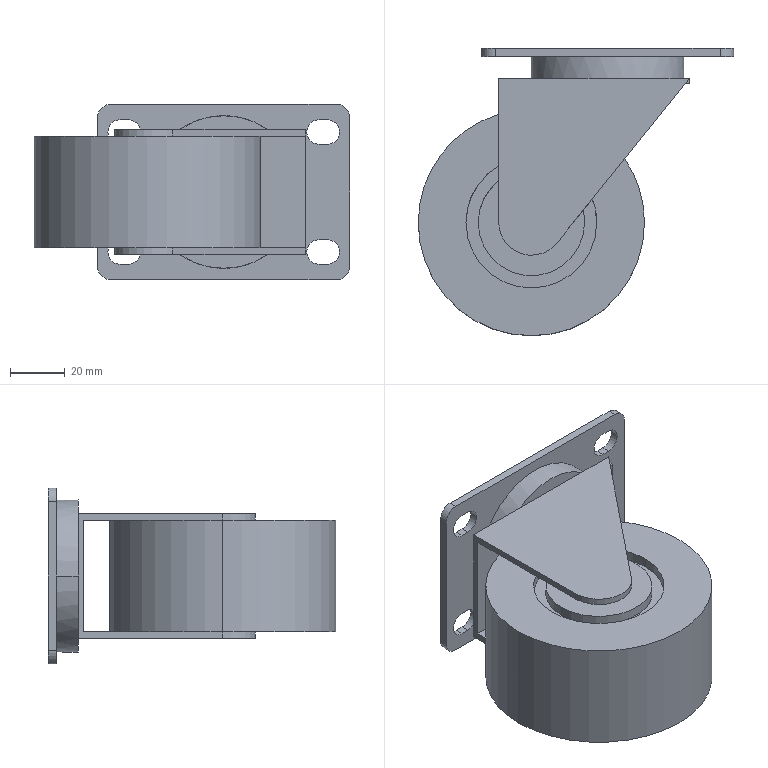Part | STEP file | universal caster-cf | 1 solid | 67 faces | box 115.75 x 105.5 x 64.5 mm | volume 273240 mm3 | plane 37 | cylinder 30 | commonest cylinder face diameters 9 x12 10 x4 39 x4 48 x4 24 x2 56 x2